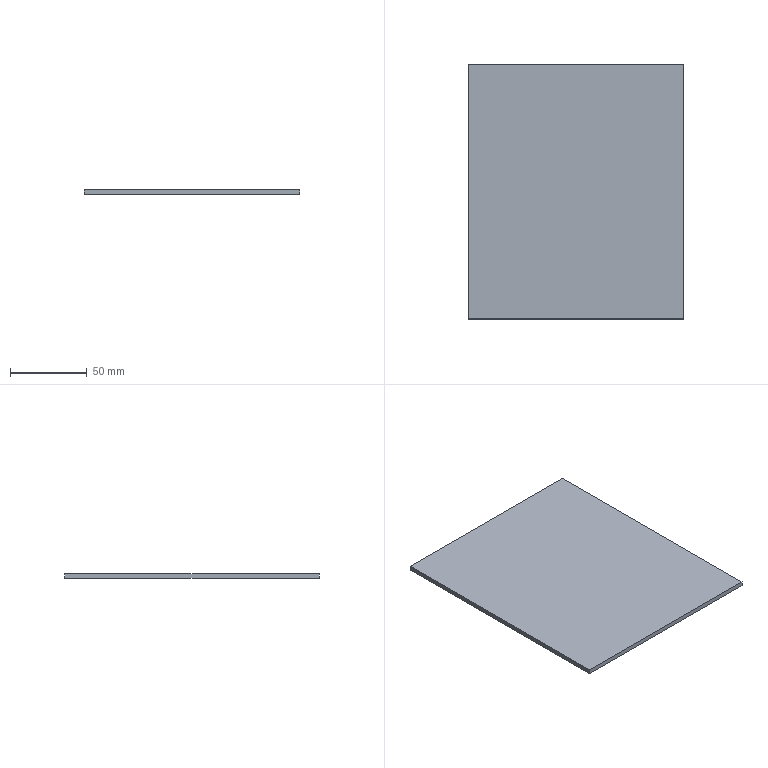Part | STEP file | 0232_A_Work | 1 solid | 6 faces | box 140 x 165 x 3 mm | volume 69300 mm3 | plane 6
STEP:
#1=CARTESIAN_POINT('',(0.,0.,0.));
#2=DIRECTION('',(0.,0.,1.));
#3=DIRECTION('',(1.,0.,0.));
#4=AXIS2_PLACEMENT_3D('',#1,#2,#3);
#5=CARTESIAN_POINT('',(-70.,165.,0.));
#6=VERTEX_POINT('',#5);
#7=CARTESIAN_POINT('',(-70.,0.,0.));
#8=VERTEX_POINT('',#7);
#9=CARTESIAN_POINT('',(-70.,165.,0.));
#10=DIRECTION('',(0.,-1.,0.));
#11=VECTOR('',#10,1.);
#12=LINE('',#9,#11);
#13=CARTESIAN_POINT('',(-70.,165.,3.));
#14=DIRECTION('',(1.,0.,0.));
#15=DIRECTION('',(0.,0.,-1.));
#16=AXIS2_PLACEMENT_3D('',#13,#14,#15);
#17=PLANE('',#16);
#18=CARTESIAN_POINT('',(3.,0.));
#19=DIRECTION('',(0.,-1.));
#20=VECTOR('',#19,1.);
#21=LINE('',#18,#20);
#22=(GEOMETRIC_REPRESENTATION_CONTEXT(2)PARAMETRIC_REPRESENTATION_CONTEXT()REPRESENTATION_CONTEXT('',''));
#23=DEFINITIONAL_REPRESENTATION('',(#21),#22);
#24=PCURVE('',#17,#23);
#25=CARTESIAN_POINT('',(-70.,0.,0.));
#26=DIRECTION('',(0.,0.,1.));
#27=DIRECTION('',(1.,0.,0.));
#28=AXIS2_PLACEMENT_3D('',#25,#26,#27);
#29=PLANE('',#28);
#30=CARTESIAN_POINT('',(0.,165.));
#31=DIRECTION('',(0.,-1.));
#32=VECTOR('',#31,1.);
#33=LINE('',#30,#32);
#34=(GEOMETRIC_REPRESENTATION_CONTEXT(2)PARAMETRIC_REPRESENTATION_CONTEXT()REPRESENTATION_CONTEXT('',''));
#35=DEFINITIONAL_REPRESENTATION('',(#33),#34);
#36=PCURVE('',#29,#35);
#37=SURFACE_CURVE('',#12,(#24,#36),.PCURVE_S1.);
#38=EDGE_CURVE('',#6,#8,#37,.T.);
#39=ORIENTED_EDGE('',*,*,#38,.T.);
#40=CARTESIAN_POINT('',(-70.,0.,3.));
#41=VERTEX_POINT('',#40);
#42=CARTESIAN_POINT('',(-70.,0.,3.));
#43=DIRECTION('',(0.,0.,-1.));
#44=VECTOR('',#43,1.);
#45=LINE('',#42,#44);
#46=CARTESIAN_POINT('',(0.,-165.));
#47=DIRECTION('',(1.,0.));
#48=VECTOR('',#47,1.);
#49=LINE('',#46,#48);
#50=(GEOMETRIC_REPRESENTATION_CONTEXT(2)PARAMETRIC_REPRESENTATION_CONTEXT()REPRESENTATION_CONTEXT('',''));
#51=DEFINITIONAL_REPRESENTATION('',(#49),#50);
#52=PCURVE('',#17,#51);
#53=CARTESIAN_POINT('',(-70.,0.,3.));
#54=DIRECTION('',(0.,1.,0.));
#55=DIRECTION('',(0.,0.,1.));
#56=AXIS2_PLACEMENT_3D('',#53,#54,#55);
#57=PLANE('',#56);
#58=CARTESIAN_POINT('',(0.,0.));
#59=DIRECTION('',(-1.,0.));
#60=VECTOR('',#59,1.);
#61=LINE('',#58,#60);
#62=(GEOMETRIC_REPRESENTATION_CONTEXT(2)PARAMETRIC_REPRESENTATION_CONTEXT()REPRESENTATION_CONTEXT('',''));
#63=DEFINITIONAL_REPRESENTATION('',(#61),#62);
#64=PCURVE('',#57,#63);
#65=SURFACE_CURVE('',#45,(#52,#64),.PCURVE_S1.);
#66=EDGE_CURVE('',#41,#8,#65,.T.);
#67=ORIENTED_EDGE('',*,*,#66,.F.);
#68=CARTESIAN_POINT('',(-70.,165.,3.));
#69=VERTEX_POINT('',#68);
#70=CARTESIAN_POINT('',(-70.,165.,3.));
#71=DIRECTION('',(0.,-1.,0.));
#72=VECTOR('',#71,1.);
#73=LINE('',#70,#72);
#74=CARTESIAN_POINT('',(0.,0.));
#75=DIRECTION('',(0.,-1.));
#76=VECTOR('',#75,1.);
#77=LINE('',#74,#76);
#78=(GEOMETRIC_REPRESENTATION_CONTEXT(2)PARAMETRIC_REPRESENTATION_CONTEXT()REPRESENTATION_CONTEXT('',''));
#79=DEFINITIONAL_REPRESENTATION('',(#77),#78);
#80=PCURVE('',#17,#79);
#81=CARTESIAN_POINT('',(-70.,0.,3.));
#82=DIRECTION('',(0.,0.,1.));
#83=DIRECTION('',(1.,0.,0.));
#84=AXIS2_PLACEMENT_3D('',#81,#82,#83);
#85=PLANE('',#84);
#86=CARTESIAN_POINT('',(0.,165.));
#87=DIRECTION('',(0.,-1.));
#88=VECTOR('',#87,1.);
#89=LINE('',#86,#88);
#90=(GEOMETRIC_REPRESENTATION_CONTEXT(2)PARAMETRIC_REPRESENTATION_CONTEXT()REPRESENTATION_CONTEXT('',''));
#91=DEFINITIONAL_REPRESENTATION('',(#89),#90);
#92=PCURVE('',#85,#91);
#93=SURFACE_CURVE('',#73,(#80,#92),.PCURVE_S1.);
#94=EDGE_CURVE('',#69,#41,#93,.T.);
#95=ORIENTED_EDGE('',*,*,#94,.F.);
#96=CARTESIAN_POINT('',(-70.,165.,3.));
#97=DIRECTION('',(0.,0.,-1.));
#98=VECTOR('',#97,1.);
#99=LINE('',#96,#98);
#100=CARTESIAN_POINT('',(0.,0.));
#101=DIRECTION('',(1.,0.));
#102=VECTOR('',#101,1.);
#103=LINE('',#100,#102);
#104=(GEOMETRIC_REPRESENTATION_CONTEXT(2)PARAMETRIC_REPRESENTATION_CONTEXT()REPRESENTATION_CONTEXT('',''));
#105=DEFINITIONAL_REPRESENTATION('',(#103),#104);
#106=PCURVE('',#17,#105);
#107=CARTESIAN_POINT('',(-70.,165.,3.));
#108=DIRECTION('',(0.,-1.,0.));
#109=DIRECTION('',(0.,0.,-1.));
#110=AXIS2_PLACEMENT_3D('',#107,#108,#109);
#111=PLANE('',#110);
#112=CARTESIAN_POINT('',(0.,0.));
#113=DIRECTION('',(1.,0.));
#114=VECTOR('',#113,1.);
#115=LINE('',#112,#114);
#116=(GEOMETRIC_REPRESENTATION_CONTEXT(2)PARAMETRIC_REPRESENTATION_CONTEXT()REPRESENTATION_CONTEXT('',''));
#117=DEFINITIONAL_REPRESENTATION('',(#115),#116);
#118=PCURVE('',#111,#117);
#119=SURFACE_CURVE('',#99,(#106,#118),.PCURVE_S1.);
#120=EDGE_CURVE('',#69,#6,#119,.T.);
#121=ORIENTED_EDGE('',*,*,#120,.T.);
#122=EDGE_LOOP('',(#39,#67,#95,#121));
#123=FACE_BOUND('',#122,.T.);
#124=ADVANCED_FACE('',(#123),#17,.F.);
#125=CARTESIAN_POINT('',(70.,0.,0.));
#126=VERTEX_POINT('',#125);
#127=CARTESIAN_POINT('',(-70.,0.,0.));
#128=DIRECTION('',(1.,0.,0.));
#129=VECTOR('',#128,1.);
#130=LINE('',#127,#129);
#131=CARTESIAN_POINT('',(-3.,0.));
#132=DIRECTION('',(0.,1.));
#133=VECTOR('',#132,1.);
#134=LINE('',#131,#133);
#135=(GEOMETRIC_REPRESENTATION_CONTEXT(2)PARAMETRIC_REPRESENTATION_CONTEXT()REPRESENTATION_CONTEXT('',''));
#136=DEFINITIONAL_REPRESENTATION('',(#134),#135);
#137=PCURVE('',#57,#136);
#138=CARTESIAN_POINT('',(0.,0.));
#139=DIRECTION('',(1.,0.));
#140=VECTOR('',#139,1.);
#141=LINE('',#138,#140);
#142=(GEOMETRIC_REPRESENTATION_CONTEXT(2)PARAMETRIC_REPRESENTATION_CONTEXT()REPRESENTATION_CONTEXT('',''));
#143=DEFINITIONAL_REPRESENTATION('',(#141),#142);
#144=PCURVE('',#29,#143);
#145=SURFACE_CURVE('',#130,(#137,#144),.PCURVE_S1.);
#146=EDGE_CURVE('',#8,#126,#145,.T.);
#147=ORIENTED_EDGE('',*,*,#146,.T.);
#148=CARTESIAN_POINT('',(70.,0.,3.));
#149=VERTEX_POINT('',#148);
#150=CARTESIAN_POINT('',(70.,0.,3.));
#151=DIRECTION('',(0.,0.,-1.));
#152=VECTOR('',#151,1.);
#153=LINE('',#150,#152);
#154=CARTESIAN_POINT('',(0.,140.));
#155=DIRECTION('',(-1.,0.));
#156=VECTOR('',#155,1.);
#157=LINE('',#154,#156);
#158=(GEOMETRIC_REPRESENTATION_CONTEXT(2)PARAMETRIC_REPRESENTATION_CONTEXT()REPRESENTATION_CONTEXT('',''));
#159=DEFINITIONAL_REPRESENTATION('',(#157),#158);
#160=PCURVE('',#57,#159);
#161=CARTESIAN_POINT('',(70.,165.,3.));
#162=DIRECTION('',(-1.,0.,0.));
#163=DIRECTION('',(0.,0.,1.));
#164=AXIS2_PLACEMENT_3D('',#161,#162,#163);
#165=PLANE('',#164);
#166=CARTESIAN_POINT('',(0.,-165.));
#167=DIRECTION('',(-1.,0.));
#168=VECTOR('',#167,1.);
#169=LINE('',#166,#168);
#170=(GEOMETRIC_REPRESENTATION_CONTEXT(2)PARAMETRIC_REPRESENTATION_CONTEXT()REPRESENTATION_CONTEXT('',''));
#171=DEFINITIONAL_REPRESENTATION('',(#169),#170);
#172=PCURVE('',#165,#171);
#173=SURFACE_CURVE('',#153,(#160,#172),.PCURVE_S1.);
#174=EDGE_CURVE('',#149,#126,#173,.T.);
#175=ORIENTED_EDGE('',*,*,#174,.F.);
#176=CARTESIAN_POINT('',(-70.,0.,3.));
#177=DIRECTION('',(1.,0.,0.));
#178=VECTOR('',#177,1.);
#179=LINE('',#176,#178);
#180=CARTESIAN_POINT('',(0.,0.));
#181=DIRECTION('',(0.,1.));
#182=VECTOR('',#181,1.);
#183=LINE('',#180,#182);
#184=(GEOMETRIC_REPRESENTATION_CONTEXT(2)PARAMETRIC_REPRESENTATION_CONTEXT()REPRESENTATION_CONTEXT('',''));
#185=DEFINITIONAL_REPRESENTATION('',(#183),#184);
#186=PCURVE('',#57,#185);
#187=CARTESIAN_POINT('',(0.,0.));
#188=DIRECTION('',(1.,0.));
#189=VECTOR('',#188,1.);
#190=LINE('',#187,#189);
#191=(GEOMETRIC_REPRESENTATION_CONTEXT(2)PARAMETRIC_REPRESENTATION_CONTEXT()REPRESENTATION_CONTEXT('',''));
#192=DEFINITIONAL_REPRESENTATION('',(#190),#191);
#193=PCURVE('',#85,#192);
#194=SURFACE_CURVE('',#179,(#186,#193),.PCURVE_S1.);
#195=EDGE_CURVE('',#41,#149,#194,.T.);
#196=ORIENTED_EDGE('',*,*,#195,.F.);
#197=ORIENTED_EDGE('',*,*,#66,.T.);
#198=EDGE_LOOP('',(#147,#175,#196,#197));
#199=FACE_BOUND('',#198,.T.);
#200=ADVANCED_FACE('',(#199),#57,.F.);
#201=CARTESIAN_POINT('',(70.,165.,0.));
#202=VERTEX_POINT('',#201);
#203=CARTESIAN_POINT('',(70.,165.,0.));
#204=DIRECTION('',(0.,1.,0.));
#205=VECTOR('',#204,1.);
#206=LINE('',#203,#205);
#207=CARTESIAN_POINT('',(-3.,0.));
#208=DIRECTION('',(0.,1.));
#209=VECTOR('',#208,1.);
#210=LINE('',#207,#209);
#211=(GEOMETRIC_REPRESENTATION_CONTEXT(2)PARAMETRIC_REPRESENTATION_CONTEXT()REPRESENTATION_CONTEXT('',''));
#212=DEFINITIONAL_REPRESENTATION('',(#210),#211);
#213=PCURVE('',#165,#212);
#214=CARTESIAN_POINT('',(140.,165.));
#215=DIRECTION('',(0.,1.));
#216=VECTOR('',#215,1.);
#217=LINE('',#214,#216);
#218=(GEOMETRIC_REPRESENTATION_CONTEXT(2)PARAMETRIC_REPRESENTATION_CONTEXT()REPRESENTATION_CONTEXT('',''));
#219=DEFINITIONAL_REPRESENTATION('',(#217),#218);
#220=PCURVE('',#29,#219);
#221=SURFACE_CURVE('',#206,(#213,#220),.PCURVE_S1.);
#222=EDGE_CURVE('',#126,#202,#221,.T.);
#223=ORIENTED_EDGE('',*,*,#222,.T.);
#224=CARTESIAN_POINT('',(70.,165.,3.));
#225=VERTEX_POINT('',#224);
#226=CARTESIAN_POINT('',(70.,165.,3.));
#227=DIRECTION('',(0.,0.,-1.));
#228=VECTOR('',#227,1.);
#229=LINE('',#226,#228);
#230=CARTESIAN_POINT('',(0.,0.));
#231=DIRECTION('',(-1.,0.));
#232=VECTOR('',#231,1.);
#233=LINE('',#230,#232);
#234=(GEOMETRIC_REPRESENTATION_CONTEXT(2)PARAMETRIC_REPRESENTATION_CONTEXT()REPRESENTATION_CONTEXT('',''));
#235=DEFINITIONAL_REPRESENTATION('',(#233),#234);
#236=PCURVE('',#165,#235);
#237=CARTESIAN_POINT('',(0.,140.));
#238=DIRECTION('',(1.,0.));
#239=VECTOR('',#238,1.);
#240=LINE('',#237,#239);
#241=(GEOMETRIC_REPRESENTATION_CONTEXT(2)PARAMETRIC_REPRESENTATION_CONTEXT()REPRESENTATION_CONTEXT('',''));
#242=DEFINITIONAL_REPRESENTATION('',(#240),#241);
#243=PCURVE('',#111,#242);
#244=SURFACE_CURVE('',#229,(#236,#243),.PCURVE_S1.);
#245=EDGE_CURVE('',#225,#202,#244,.T.);
#246=ORIENTED_EDGE('',*,*,#245,.F.);
#247=CARTESIAN_POINT('',(70.,165.,3.));
#248=DIRECTION('',(0.,1.,0.));
#249=VECTOR('',#248,1.);
#250=LINE('',#247,#249);
#251=CARTESIAN_POINT('',(0.,0.));
#252=DIRECTION('',(0.,1.));
#253=VECTOR('',#252,1.);
#254=LINE('',#251,#253);
#255=(GEOMETRIC_REPRESENTATION_CONTEXT(2)PARAMETRIC_REPRESENTATION_CONTEXT()REPRESENTATION_CONTEXT('',''));
#256=DEFINITIONAL_REPRESENTATION('',(#254),#255);
#257=PCURVE('',#165,#256);
#258=CARTESIAN_POINT('',(140.,165.));
#259=DIRECTION('',(0.,1.));
#260=VECTOR('',#259,1.);
#261=LINE('',#258,#260);
#262=(GEOMETRIC_REPRESENTATION_CONTEXT(2)PARAMETRIC_REPRESENTATION_CONTEXT()REPRESENTATION_CONTEXT('',''));
#263=DEFINITIONAL_REPRESENTATION('',(#261),#262);
#264=PCURVE('',#85,#263);
#265=SURFACE_CURVE('',#250,(#257,#264),.PCURVE_S1.);
#266=EDGE_CURVE('',#149,#225,#265,.T.);
#267=ORIENTED_EDGE('',*,*,#266,.F.);
#268=ORIENTED_EDGE('',*,*,#174,.T.);
#269=EDGE_LOOP('',(#223,#246,#267,#268));
#270=FACE_BOUND('',#269,.T.);
#271=ADVANCED_FACE('',(#270),#165,.F.);
#272=CARTESIAN_POINT('',(-70.,165.,0.));
#273=DIRECTION('',(-1.,0.,0.));
#274=VECTOR('',#273,1.);
#275=LINE('',#272,#274);
#276=CARTESIAN_POINT('',(3.,0.));
#277=DIRECTION('',(0.,-1.));
#278=VECTOR('',#277,1.);
#279=LINE('',#276,#278);
#280=(GEOMETRIC_REPRESENTATION_CONTEXT(2)PARAMETRIC_REPRESENTATION_CONTEXT()REPRESENTATION_CONTEXT('',''));
#281=DEFINITIONAL_REPRESENTATION('',(#279),#280);
#282=PCURVE('',#111,#281);
#283=CARTESIAN_POINT('',(0.,165.));
#284=DIRECTION('',(-1.,0.));
#285=VECTOR('',#284,1.);
#286=LINE('',#283,#285);
#287=(GEOMETRIC_REPRESENTATION_CONTEXT(2)PARAMETRIC_REPRESENTATION_CONTEXT()REPRESENTATION_CONTEXT('',''));
#288=DEFINITIONAL_REPRESENTATION('',(#286),#287);
#289=PCURVE('',#29,#288);
#290=SURFACE_CURVE('',#275,(#282,#289),.PCURVE_S1.);
#291=EDGE_CURVE('',#202,#6,#290,.T.);
#292=ORIENTED_EDGE('',*,*,#291,.T.);
#293=ORIENTED_EDGE('',*,*,#120,.F.);
#294=CARTESIAN_POINT('',(-70.,165.,3.));
#295=DIRECTION('',(-1.,0.,0.));
#296=VECTOR('',#295,1.);
#297=LINE('',#294,#296);
#298=CARTESIAN_POINT('',(0.,0.));
#299=DIRECTION('',(0.,-1.));
#300=VECTOR('',#299,1.);
#301=LINE('',#298,#300);
#302=(GEOMETRIC_REPRESENTATION_CONTEXT(2)PARAMETRIC_REPRESENTATION_CONTEXT()REPRESENTATION_CONTEXT('',''));
#303=DEFINITIONAL_REPRESENTATION('',(#301),#302);
#304=PCURVE('',#111,#303);
#305=CARTESIAN_POINT('',(0.,165.));
#306=DIRECTION('',(-1.,0.));
#307=VECTOR('',#306,1.);
#308=LINE('',#305,#307);
#309=(GEOMETRIC_REPRESENTATION_CONTEXT(2)PARAMETRIC_REPRESENTATION_CONTEXT()REPRESENTATION_CONTEXT('',''));
#310=DEFINITIONAL_REPRESENTATION('',(#308),#309);
#311=PCURVE('',#85,#310);
#312=SURFACE_CURVE('',#297,(#304,#311),.PCURVE_S1.);
#313=EDGE_CURVE('',#225,#69,#312,.T.);
#314=ORIENTED_EDGE('',*,*,#313,.F.);
#315=ORIENTED_EDGE('',*,*,#245,.T.);
#316=EDGE_LOOP('',(#292,#293,#314,#315));
#317=FACE_BOUND('',#316,.T.);
#318=ADVANCED_FACE('',(#317),#111,.F.);
#319=ORIENTED_EDGE('',*,*,#94,.T.);
#320=ORIENTED_EDGE('',*,*,#195,.T.);
#321=ORIENTED_EDGE('',*,*,#266,.T.);
#322=ORIENTED_EDGE('',*,*,#313,.T.);
#323=EDGE_LOOP('',(#319,#320,#321,#322));
#324=FACE_BOUND('',#323,.T.);
#325=ADVANCED_FACE('',(#324),#85,.T.);
#326=ORIENTED_EDGE('',*,*,#38,.F.);
#327=ORIENTED_EDGE('',*,*,#291,.F.);
#328=ORIENTED_EDGE('',*,*,#222,.F.);
#329=ORIENTED_EDGE('',*,*,#146,.F.);
#330=EDGE_LOOP('',(#326,#327,#328,#329));
#331=FACE_BOUND('',#330,.T.);
#332=ADVANCED_FACE('',(#331),#29,.F.);
#333=CLOSED_SHELL('',(#124,#200,#271,#318,#325,#332));
#334=MANIFOLD_SOLID_BREP('',#333);
#335=(LENGTH_UNIT()NAMED_UNIT(*)SI_UNIT(.MILLI.,.METRE.));
#336=UNCERTAINTY_MEASURE_WITH_UNIT(LENGTH_MEASURE(0.0000001),#335,'','');
#337=(NAMED_UNIT(*)PLANE_ANGLE_UNIT()SI_UNIT($,.RADIAN.));
#338=(NAMED_UNIT(*)SI_UNIT($,.STERADIAN.)SOLID_ANGLE_UNIT());
#339=(GEOMETRIC_REPRESENTATION_CONTEXT(3)GLOBAL_UNCERTAINTY_ASSIGNED_CONTEXT((#336))GLOBAL_UNIT_ASSIGNED_CONTEXT((#335,#337,#338))REPRESENTATION_CONTEXT('',''));
#340=ADVANCED_BREP_SHAPE_REPRESENTATION('',(#4,#334),#339);